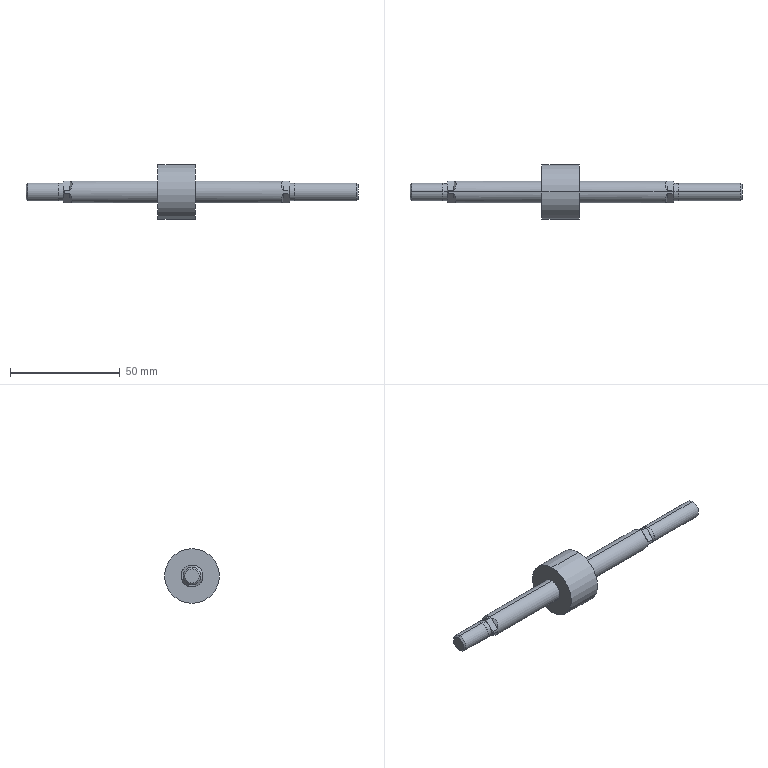Part | STEP file | 001-008-_SDAJS-25x30-B1030_r | 1 solid | 52 faces | box 151 x 24.9 x 24.9 mm | volume 17310 mm3 | plane 24 | cylinder 14 | cone 14 | commonest cylinder face diameters 7.8 x4 8 x4 10 x4 24.9 x2